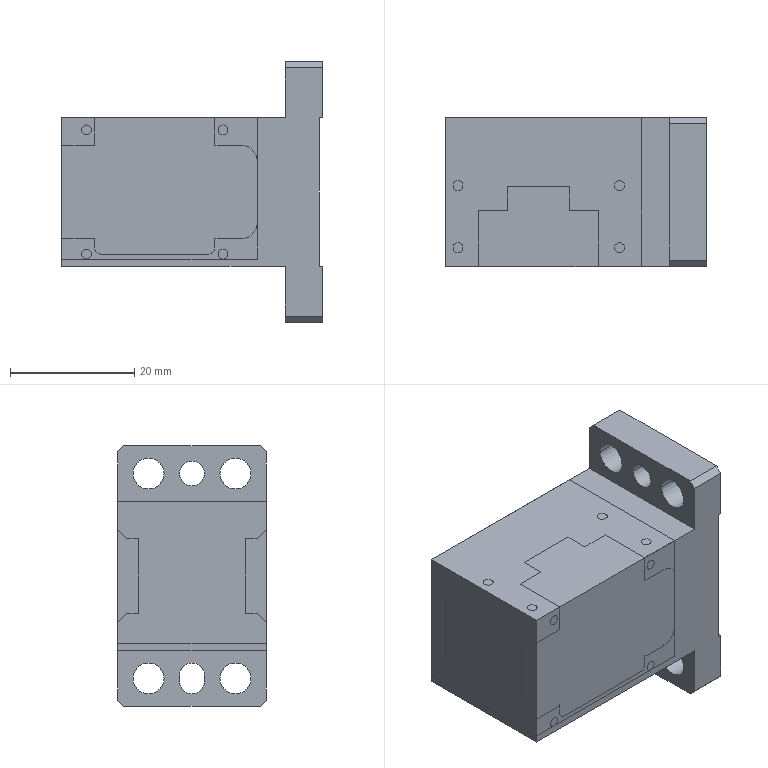Part | 2 solids | 152 faces | box 42 x 24 x 42 mm | volume 32864 mm3 | plane 60 | cylinder 56 | cone 36 | commonest cylinder face diameters 1.6 x32 2 x12 5 x8 4 x4